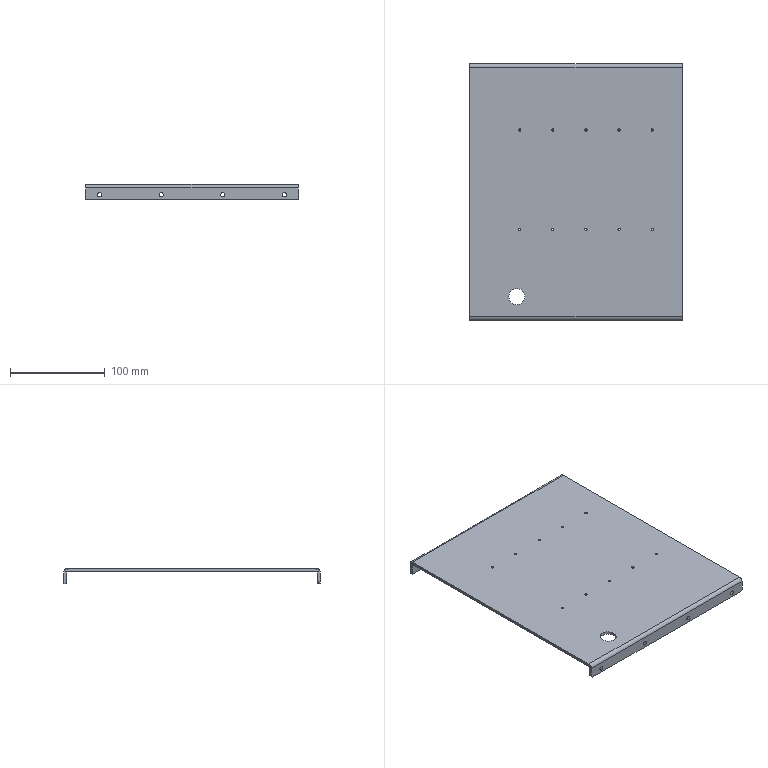Part | STEP file | GLSJ-10-38 | 1 solid | 62 faces | box 225 x 271 x 16 mm | volume 197957 mm3 | cylinder 42 | plane 20 | commonest cylinder face diameters 2.5 x20 4.5 x16 1.473 x2 7.473 x2 17 x2